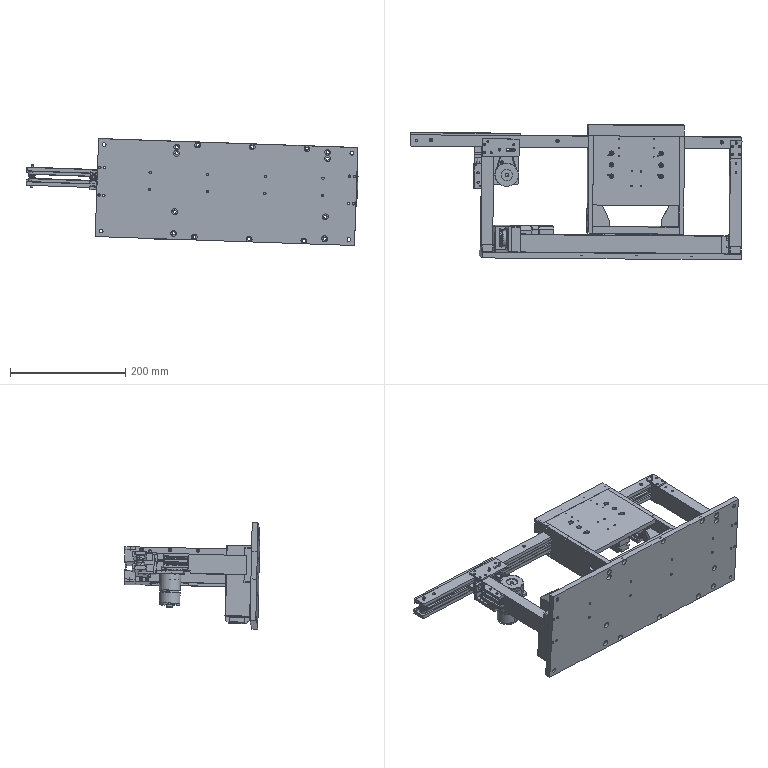Part | SolidWorks | 77 solids | 2628 faces | box 575.911 x 235.705 x 185.668 mm | volume 2678930 mm3 | cylinder 1334 | plane 961 | cone 310 | spline 19 | torus 4 | commonest cylinder face diameters 2.459 x206 3.5 x162 6 x130 5.5 x112 10 x98 4.134 x80